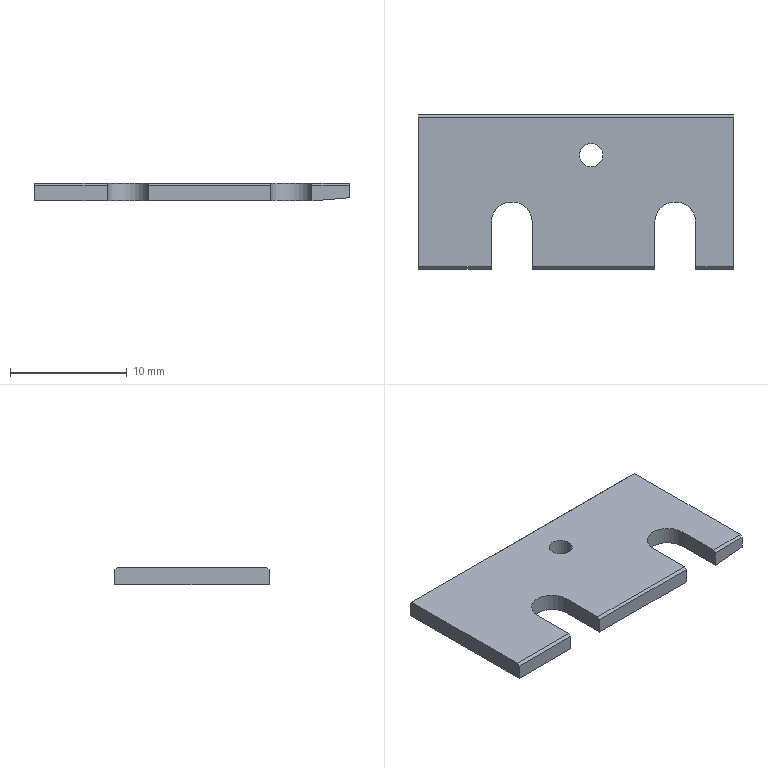Part | NX | 1 solid | 21 faces | box 27 x 13.2 x 1.5 mm | volume 467.319 mm3 | plane 17 | cylinder 4 | commonest cylinder face diameters 2 x2 3.5 x2
STEP:
#1=CARTESIAN_POINT('',(10.25,-7.3,0.75));
#2=VERTEX_POINT('',#1);
#3=CARTESIAN_POINT('',(13.5,-7.3,0.75));
#4=VERTEX_POINT('',#3);
#5=CARTESIAN_POINT('',(0.,-7.3,0.75));
#6=DIRECTION('',(1.,0.,0.));
#7=VECTOR('',#6,1000.);
#8=LINE('',#5,#7);
#9=EDGE_CURVE('',#2,#4,#8,.T.);
#10=ORIENTED_EDGE('',*,*,#9,.T.);
#11=CARTESIAN_POINT('',(13.5,5.5,0.75));
#12=VERTEX_POINT('',#11);
#13=CARTESIAN_POINT('',(13.5,0.,0.75));
#14=DIRECTION('',(0.,-1.,0.));
#15=VECTOR('',#14,1000.);
#16=LINE('',#13,#15);
#17=EDGE_CURVE('',#12,#4,#16,.T.);
#18=ORIENTED_EDGE('',*,*,#17,.F.);
#19=CARTESIAN_POINT('',(-13.5,5.5,0.75));
#20=VERTEX_POINT('',#19);
#21=CARTESIAN_POINT('',(0.,5.5,0.75));
#22=DIRECTION('',(-1.,0.,0.));
#23=VECTOR('',#22,1000.);
#24=LINE('',#21,#23);
#25=EDGE_CURVE('',#12,#20,#24,.T.);
#26=ORIENTED_EDGE('',*,*,#25,.T.);
#27=CARTESIAN_POINT('',(-13.5,-7.3,0.75));
#28=VERTEX_POINT('',#27);
#29=CARTESIAN_POINT('',(-13.5,0.,0.75));
#30=DIRECTION('',(0.,1.,0.));
#31=VECTOR('',#30,1000.);
#32=LINE('',#29,#31);
#33=EDGE_CURVE('',#28,#20,#32,.T.);
#34=ORIENTED_EDGE('',*,*,#33,.F.);
#35=CARTESIAN_POINT('',(-7.25,-7.3,0.75));
#36=VERTEX_POINT('',#35);
#37=CARTESIAN_POINT('',(0.,-7.3,0.75));
#38=DIRECTION('',(1.,0.,0.));
#39=VECTOR('',#38,1000.);
#40=LINE('',#37,#39);
#41=EDGE_CURVE('',#28,#36,#40,.T.);
#42=ORIENTED_EDGE('',*,*,#41,.T.);
#43=CARTESIAN_POINT('',(-7.25,-3.5,0.75));
#44=VERTEX_POINT('',#43);
#45=CARTESIAN_POINT('',(-7.25,0.,0.75));
#46=DIRECTION('',(0.,1.,0.));
#47=VECTOR('',#46,1000.);
#48=LINE('',#45,#47);
#49=EDGE_CURVE('',#36,#44,#48,.T.);
#50=ORIENTED_EDGE('',*,*,#49,.T.);
#51=CARTESIAN_POINT('',(-3.75,-3.5,0.75));
#52=VERTEX_POINT('',#51);
#53=CARTESIAN_POINT('',(-5.5,-3.5,0.75));
#54=DIRECTION('',(0.,0.,-1.));
#55=DIRECTION('',(-1.,0.,0.));
#56=AXIS2_PLACEMENT_3D('',#53,#54,#55);
#57=CIRCLE('',#56,1.75);
#58=EDGE_CURVE('',#44,#52,#57,.T.);
#59=ORIENTED_EDGE('',*,*,#58,.T.);
#60=CARTESIAN_POINT('',(-3.75,-7.3,0.75));
#61=VERTEX_POINT('',#60);
#62=CARTESIAN_POINT('',(-3.75,0.,0.75));
#63=DIRECTION('',(0.,-1.,0.));
#64=VECTOR('',#63,1000.);
#65=LINE('',#62,#64);
#66=EDGE_CURVE('',#52,#61,#65,.T.);
#67=ORIENTED_EDGE('',*,*,#66,.T.);
#68=CARTESIAN_POINT('',(6.75,-7.3,0.75));
#69=VERTEX_POINT('',#68);
#70=CARTESIAN_POINT('',(0.,-7.3,0.75));
#71=DIRECTION('',(1.,0.,0.));
#72=VECTOR('',#71,1000.);
#73=LINE('',#70,#72);
#74=EDGE_CURVE('',#61,#69,#73,.T.);
#75=ORIENTED_EDGE('',*,*,#74,.T.);
#76=CARTESIAN_POINT('',(6.75,-3.5,0.75));
#77=VERTEX_POINT('',#76);
#78=CARTESIAN_POINT('',(6.75,0.,0.75));
#79=DIRECTION('',(0.,1.,0.));
#80=VECTOR('',#79,1000.);
#81=LINE('',#78,#80);
#82=EDGE_CURVE('',#69,#77,#81,.T.);
#83=ORIENTED_EDGE('',*,*,#82,.T.);
#84=CARTESIAN_POINT('',(10.25,-3.5,0.75));
#85=VERTEX_POINT('',#84);
#86=CARTESIAN_POINT('',(8.5,-3.5,0.75));
#87=DIRECTION('',(0.,0.,-1.));
#88=DIRECTION('',(-1.,0.,0.));
#89=AXIS2_PLACEMENT_3D('',#86,#87,#88);
#90=CIRCLE('',#89,1.75);
#91=EDGE_CURVE('',#77,#85,#90,.T.);
#92=ORIENTED_EDGE('',*,*,#91,.T.);
#93=CARTESIAN_POINT('',(10.25,0.,0.75));
#94=DIRECTION('',(0.,-1.,0.));
#95=VECTOR('',#94,1000.);
#96=LINE('',#93,#95);
#97=EDGE_CURVE('',#85,#2,#96,.T.);
#98=ORIENTED_EDGE('',*,*,#97,.T.);
#99=EDGE_LOOP('',(#10,#18,#26,#34,#42,#50,#59,#67,#75,#83,#92,#98));
#100=FACE_BOUND('',#99,.T.);
#101=CARTESIAN_POINT('',(0.3,2.25,0.75));
#102=VERTEX_POINT('',#101);
#103=CARTESIAN_POINT('',(2.3,2.25,0.75));
#104=VERTEX_POINT('',#103);
#105=CARTESIAN_POINT('',(1.3,2.25,0.75));
#106=DIRECTION('',(0.,0.,-1.));
#107=DIRECTION('',(-1.,0.,0.));
#108=AXIS2_PLACEMENT_3D('',#105,#106,#107);
#109=CIRCLE('',#108,1.);
#110=EDGE_CURVE('',#102,#104,#109,.T.);
#111=ORIENTED_EDGE('',*,*,#110,.T.);
#112=CARTESIAN_POINT('',(1.3,2.25,0.75));
#113=DIRECTION('',(0.,0.,-1.));
#114=DIRECTION('',(-1.,0.,0.));
#115=AXIS2_PLACEMENT_3D('',#112,#113,#114);
#116=CIRCLE('',#115,1.);
#117=EDGE_CURVE('',#104,#102,#116,.T.);
#118=ORIENTED_EDGE('',*,*,#117,.T.);
#119=EDGE_LOOP('',(#111,#118));
#120=FACE_BOUND('',#119,.T.);
#121=CARTESIAN_POINT('',(0.,0.,0.75));
#122=DIRECTION('',(0.,0.,1.));
#123=DIRECTION('',(1.,0.,0.));
#124=AXIS2_PLACEMENT_3D('',#121,#122,#123);
#125=PLANE('',#124);
#126=ADVANCED_FACE('',(#100,#120),#125,.T.);
#127=CARTESIAN_POINT('',(-13.5,-7.5,-0.75));
#128=VERTEX_POINT('',#127);
#129=CARTESIAN_POINT('',(-13.5,5.7,-0.75));
#130=VERTEX_POINT('',#129);
#131=CARTESIAN_POINT('',(-13.5,0.,-0.75));
#132=DIRECTION('',(0.,1.,0.));
#133=VECTOR('',#132,1000.);
#134=LINE('',#131,#133);
#135=EDGE_CURVE('',#128,#130,#134,.T.);
#136=ORIENTED_EDGE('',*,*,#135,.F.);
#137=CARTESIAN_POINT('',(-13.5,-7.5,0.55));
#138=VERTEX_POINT('',#137);
#139=CARTESIAN_POINT('',(-13.5,-7.5,0.));
#140=DIRECTION('',(0.,0.,-1.));
#141=VECTOR('',#140,1000.);
#142=LINE('',#139,#141);
#143=EDGE_CURVE('',#138,#128,#142,.T.);
#144=ORIENTED_EDGE('',*,*,#143,.F.);
#145=CARTESIAN_POINT('',(-13.5,0.,8.05));
#146=DIRECTION('',(0.,0.7071,0.7071));
#147=VECTOR('',#146,1000.);
#148=LINE('',#145,#147);
#149=EDGE_CURVE('',#138,#28,#148,.T.);
#150=ORIENTED_EDGE('',*,*,#149,.T.);
#151=ORIENTED_EDGE('',*,*,#33,.T.);
#152=CARTESIAN_POINT('',(-13.5,5.7,0.55));
#153=VERTEX_POINT('',#152);
#154=CARTESIAN_POINT('',(-13.5,0.,6.25));
#155=DIRECTION('',(0.,0.7071,-0.7071));
#156=VECTOR('',#155,1000.);
#157=LINE('',#154,#156);
#158=EDGE_CURVE('',#20,#153,#157,.T.);
#159=ORIENTED_EDGE('',*,*,#158,.T.);
#160=CARTESIAN_POINT('',(-13.5,5.7,0.));
#161=DIRECTION('',(0.,0.,-1.));
#162=VECTOR('',#161,1000.);
#163=LINE('',#160,#162);
#164=EDGE_CURVE('',#153,#130,#163,.T.);
#165=ORIENTED_EDGE('',*,*,#164,.T.);
#166=EDGE_LOOP('',(#136,#144,#150,#151,#159,#165));
#167=FACE_BOUND('',#166,.T.);
#168=CARTESIAN_POINT('',(-13.5,7.5,-0.75));
#169=DIRECTION('',(-1.,0.,0.));
#170=DIRECTION('',(0.,0.,1.));
#171=AXIS2_PLACEMENT_3D('',#168,#169,#170);
#172=PLANE('',#171);
#173=ADVANCED_FACE('',(#167),#172,.T.);
#174=CARTESIAN_POINT('',(10.5,5.7,-0.75));
#175=VERTEX_POINT('',#174);
#176=CARTESIAN_POINT('',(0.,5.7,-0.75));
#177=DIRECTION('',(1.,0.,0.));
#178=VECTOR('',#177,1000.);
#179=LINE('',#176,#178);
#180=EDGE_CURVE('',#130,#175,#179,.T.);
#181=ORIENTED_EDGE('',*,*,#180,.F.);
#182=ORIENTED_EDGE('',*,*,#164,.F.);
#183=CARTESIAN_POINT('',(13.5,5.7,0.55));
#184=VERTEX_POINT('',#183);
#185=CARTESIAN_POINT('',(0.,5.7,0.55));
#186=DIRECTION('',(1.,0.,0.));
#187=VECTOR('',#186,1000.);
#188=LINE('',#185,#187);
#189=EDGE_CURVE('',#153,#184,#188,.T.);
#190=ORIENTED_EDGE('',*,*,#189,.T.);
#191=CARTESIAN_POINT('',(13.5,5.7,-0.4875));
#192=VERTEX_POINT('',#191);
#193=CARTESIAN_POINT('',(13.5,5.7,0.));
#194=DIRECTION('',(0.,0.,1.));
#195=VECTOR('',#194,1000.);
#196=LINE('',#193,#195);
#197=EDGE_CURVE('',#192,#184,#196,.T.);
#198=ORIENTED_EDGE('',*,*,#197,.F.);
#199=CARTESIAN_POINT('',(0.,5.7,-1.669));
#200=DIRECTION('',(0.9962,0.,0.08716));
#201=VECTOR('',#200,1000.);
#202=LINE('',#199,#201);
#203=EDGE_CURVE('',#175,#192,#202,.T.);
#204=ORIENTED_EDGE('',*,*,#203,.F.);
#205=EDGE_LOOP('',(#181,#182,#190,#198,#204));
#206=FACE_BOUND('',#205,.T.);
#207=CARTESIAN_POINT('',(13.5,5.7,-0.75));
#208=DIRECTION('',(0.,1.,0.));
#209=DIRECTION('',(1.,0.,0.));
#210=AXIS2_PLACEMENT_3D('',#207,#208,#209);
#211=PLANE('',#210);
#212=ADVANCED_FACE('',(#206),#211,.T.);
#213=CARTESIAN_POINT('',(10.5,-7.5,-0.75));
#214=VERTEX_POINT('',#213);
#215=CARTESIAN_POINT('',(10.5,0.,-0.75));
#216=DIRECTION('',(0.,-1.,0.));
#217=VECTOR('',#216,1000.);
#218=LINE('',#215,#217);
#219=EDGE_CURVE('',#175,#214,#218,.T.);
#220=ORIENTED_EDGE('',*,*,#219,.F.);
#221=ORIENTED_EDGE('',*,*,#203,.T.);
#222=CARTESIAN_POINT('',(13.5,-7.5,-0.4875));
#223=VERTEX_POINT('',#222);
#224=CARTESIAN_POINT('',(13.5,0.,-0.4875));
#225=DIRECTION('',(0.,-1.,0.));
#226=VECTOR('',#225,1000.);
#227=LINE('',#224,#226);
#228=EDGE_CURVE('',#192,#223,#227,.T.);
#229=ORIENTED_EDGE('',*,*,#228,.T.);
#230=CARTESIAN_POINT('',(0.,-7.5,-1.669));
#231=DIRECTION('',(0.9962,0.,0.08716));
#232=VECTOR('',#231,1000.);
#233=LINE('',#230,#232);
#234=EDGE_CURVE('',#214,#223,#233,.T.);
#235=ORIENTED_EDGE('',*,*,#234,.F.);
#236=EDGE_LOOP('',(#220,#221,#229,#235));
#237=FACE_BOUND('',#236,.T.);
#238=CARTESIAN_POINT('',(10.5,-7.5,-0.75));
#239=DIRECTION('',(0.08716,0.,-0.9962));
#240=DIRECTION('',(0.,-1.,0.));
#241=AXIS2_PLACEMENT_3D('',#238,#239,#240);
#242=PLANE('',#241);
#243=ADVANCED_FACE('',(#237),#242,.T.);
#244=CARTESIAN_POINT('',(-7.25,-7.5,-0.75));
#245=VERTEX_POINT('',#244);
#246=CARTESIAN_POINT('',(0.,-7.5,-0.75));
#247=DIRECTION('',(-1.,0.,0.));
#248=VECTOR('',#247,1000.);
#249=LINE('',#246,#248);
#250=EDGE_CURVE('',#245,#128,#249,.T.);
#251=ORIENTED_EDGE('',*,*,#250,.F.);
#252=CARTESIAN_POINT('',(-7.25,-7.5,0.55));
#253=VERTEX_POINT('',#252);
#254=CARTESIAN_POINT('',(-7.25,-7.5,0.));
#255=DIRECTION('',(0.,0.,-1.));
#256=VECTOR('',#255,1000.);
#257=LINE('',#254,#256);
#258=EDGE_CURVE('',#253,#245,#257,.T.);
#259=ORIENTED_EDGE('',*,*,#258,.F.);
#260=CARTESIAN_POINT('',(0.,-7.5,0.55));
#261=DIRECTION('',(-1.,0.,0.));
#262=VECTOR('',#261,1000.);
#263=LINE('',#260,#262);
#264=EDGE_CURVE('',#253,#138,#263,.T.);
#265=ORIENTED_EDGE('',*,*,#264,.T.);
#266=ORIENTED_EDGE('',*,*,#143,.T.);
#267=EDGE_LOOP('',(#251,#259,#265,#266));
#268=FACE_BOUND('',#267,.T.);
#269=CARTESIAN_POINT('',(-13.5,-7.5,-0.75));
#270=DIRECTION('',(0.,-1.,0.));
#271=DIRECTION('',(0.,0.,-1.));
#272=AXIS2_PLACEMENT_3D('',#269,#270,#271);
#273=PLANE('',#272);
#274=ADVANCED_FACE('',(#268),#273,.T.);
#275=ORIENTED_EDGE('',*,*,#135,.T.);
#276=ORIENTED_EDGE('',*,*,#180,.T.);
#277=ORIENTED_EDGE('',*,*,#219,.T.);
#278=CARTESIAN_POINT('',(10.25,-7.5,-0.75));
#279=VERTEX_POINT('',#278);
#280=CARTESIAN_POINT('',(0.,-7.5,-0.75));
#281=DIRECTION('',(-1.,0.,0.));
#282=VECTOR('',#281,1000.);
#283=LINE('',#280,#282);
#284=EDGE_CURVE('',#214,#279,#283,.T.);
#285=ORIENTED_EDGE('',*,*,#284,.T.);
#286=CARTESIAN_POINT('',(10.25,-3.5,-0.75));
#287=VERTEX_POINT('',#286);
#288=CARTESIAN_POINT('',(10.25,0.,-0.75));
#289=DIRECTION('',(0.,-1.,0.));
#290=VECTOR('',#289,1000.);
#291=LINE('',#288,#290);
#292=EDGE_CURVE('',#287,#279,#291,.T.);
#293=ORIENTED_EDGE('',*,*,#292,.F.);
#294=CARTESIAN_POINT('',(6.75,-3.5,-0.75));
#295=VERTEX_POINT('',#294);
#296=CARTESIAN_POINT('',(8.5,-3.5,-0.75));
#297=DIRECTION('',(0.,0.,-1.));
#298=DIRECTION('',(-1.,0.,0.));
#299=AXIS2_PLACEMENT_3D('',#296,#297,#298);
#300=CIRCLE('',#299,1.75);
#301=EDGE_CURVE('',#295,#287,#300,.T.);
#302=ORIENTED_EDGE('',*,*,#301,.F.);
#303=CARTESIAN_POINT('',(6.75,-7.5,-0.75));
#304=VERTEX_POINT('',#303);
#305=CARTESIAN_POINT('',(6.75,0.,-0.75));
#306=DIRECTION('',(0.,1.,0.));
#307=VECTOR('',#306,1000.);
#308=LINE('',#305,#307);
#309=EDGE_CURVE('',#304,#295,#308,.T.);
#310=ORIENTED_EDGE('',*,*,#309,.F.);
#311=CARTESIAN_POINT('',(-3.75,-7.5,-0.75));
#312=VERTEX_POINT('',#311);
#313=CARTESIAN_POINT('',(0.,-7.5,-0.75));
#314=DIRECTION('',(-1.,0.,0.));
#315=VECTOR('',#314,1000.);
#316=LINE('',#313,#315);
#317=EDGE_CURVE('',#304,#312,#316,.T.);
#318=ORIENTED_EDGE('',*,*,#317,.T.);
#319=CARTESIAN_POINT('',(-3.75,-3.5,-0.75));
#320=VERTEX_POINT('',#319);
#321=CARTESIAN_POINT('',(-3.75,0.,-0.75));
#322=DIRECTION('',(0.,-1.,0.));
#323=VECTOR('',#322,1000.);
#324=LINE('',#321,#323);
#325=EDGE_CURVE('',#320,#312,#324,.T.);
#326=ORIENTED_EDGE('',*,*,#325,.F.);
#327=CARTESIAN_POINT('',(-7.25,-3.5,-0.75));
#328=VERTEX_POINT('',#327);
#329=CARTESIAN_POINT('',(-5.5,-3.5,-0.75));
#330=DIRECTION('',(0.,0.,-1.));
#331=DIRECTION('',(-1.,0.,0.));
#332=AXIS2_PLACEMENT_3D('',#329,#330,#331);
#333=CIRCLE('',#332,1.75);
#334=EDGE_CURVE('',#328,#320,#333,.T.);
#335=ORIENTED_EDGE('',*,*,#334,.F.);
#336=CARTESIAN_POINT('',(-7.25,0.,-0.75));
#337=DIRECTION('',(0.,1.,0.));
#338=VECTOR('',#337,1000.);
#339=LINE('',#336,#338);
#340=EDGE_CURVE('',#245,#328,#339,.T.);
#341=ORIENTED_EDGE('',*,*,#340,.F.);
#342=ORIENTED_EDGE('',*,*,#250,.T.);
#343=EDGE_LOOP('',(#275,#276,#277,#285,#293,#302,#310,#318,#326,#335,#341,#342));
#344=FACE_BOUND('',#343,.T.);
#345=CARTESIAN_POINT('',(2.3,2.25,-0.75));
#346=VERTEX_POINT('',#345);
#347=CARTESIAN_POINT('',(0.3,2.25,-0.75));
#348=VERTEX_POINT('',#347);
#349=CARTESIAN_POINT('',(1.3,2.25,-0.75));
#350=DIRECTION('',(0.,0.,-1.));
#351=DIRECTION('',(-1.,0.,0.));
#352=AXIS2_PLACEMENT_3D('',#349,#350,#351);
#353=CIRCLE('',#352,1.);
#354=EDGE_CURVE('',#346,#348,#353,.T.);
#355=ORIENTED_EDGE('',*,*,#354,.F.);
#356=CARTESIAN_POINT('',(1.3,2.25,-0.75));
#357=DIRECTION('',(0.,0.,-1.));
#358=DIRECTION('',(-1.,0.,0.));
#359=AXIS2_PLACEMENT_3D('',#356,#357,#358);
#360=CIRCLE('',#359,1.);
#361=EDGE_CURVE('',#348,#346,#360,.T.);
#362=ORIENTED_EDGE('',*,*,#361,.F.);
#363=EDGE_LOOP('',(#355,#362));
#364=FACE_BOUND('',#363,.T.);
#365=CARTESIAN_POINT('',(0.,0.,-0.75));
#366=DIRECTION('',(0.,0.,1.));
#367=DIRECTION('',(1.,0.,0.));
#368=AXIS2_PLACEMENT_3D('',#365,#366,#367);
#369=PLANE('',#368);
#370=ADVANCED_FACE('',(#344,#364),#369,.F.);
#371=ORIENTED_EDGE('',*,*,#228,.F.);
#372=ORIENTED_EDGE('',*,*,#197,.T.);
#373=CARTESIAN_POINT('',(13.5,0.,6.25));
#374=DIRECTION('',(0.,-0.7071,0.7071));
#375=VECTOR('',#374,1000.);
#376=LINE('',#373,#375);
#377=EDGE_CURVE('',#184,#12,#376,.T.);
#378=ORIENTED_EDGE('',*,*,#377,.T.);
#379=ORIENTED_EDGE('',*,*,#17,.T.);
#380=CARTESIAN_POINT('',(13.5,-7.5,0.55));
#381=VERTEX_POINT('',#380);
#382=CARTESIAN_POINT('',(13.5,0.,8.05));
#383=DIRECTION('',(0.,-0.7071,-0.7071));
#384=VECTOR('',#383,1000.);
#385=LINE('',#382,#384);
#386=EDGE_CURVE('',#4,#381,#385,.T.);
#387=ORIENTED_EDGE('',*,*,#386,.T.);
#388=CARTESIAN_POINT('',(13.5,-7.5,0.));
#389=DIRECTION('',(0.,0.,1.));
#390=VECTOR('',#389,1000.);
#391=LINE('',#388,#390);
#392=EDGE_CURVE('',#223,#381,#391,.T.);
#393=ORIENTED_EDGE('',*,*,#392,.F.);
#394=EDGE_LOOP('',(#371,#372,#378,#379,#387,#393));
#395=FACE_BOUND('',#394,.T.);
#396=CARTESIAN_POINT('',(13.5,-7.5,-0.75));
#397=DIRECTION('',(1.,0.,0.));
#398=DIRECTION('',(0.,1.,0.));
#399=AXIS2_PLACEMENT_3D('',#396,#397,#398);
#400=PLANE('',#399);
#401=ADVANCED_FACE('',(#395),#400,.T.);
#402=CARTESIAN_POINT('',(10.25,-7.5,0.55));
#403=VERTEX_POINT('',#402);
#404=CARTESIAN_POINT('',(10.25,-7.5,0.));
#405=DIRECTION('',(0.,0.,1.));
#406=VECTOR('',#405,1000.);
#407=LINE('',#404,#406);
#408=EDGE_CURVE('',#279,#403,#407,.T.);
#409=ORIENTED_EDGE('',*,*,#408,.F.);
#410=ORIENTED_EDGE('',*,*,#284,.F.);
#411=ORIENTED_EDGE('',*,*,#234,.T.);
#412=ORIENTED_EDGE('',*,*,#392,.T.);
#413=CARTESIAN_POINT('',(0.,-7.5,0.55));
#414=DIRECTION('',(-1.,0.,0.));
#415=VECTOR('',#414,1000.);
#416=LINE('',#413,#415);
#417=EDGE_CURVE('',#381,#403,#416,.T.);
#418=ORIENTED_EDGE('',*,*,#417,.T.);
#419=EDGE_LOOP('',(#409,#410,#411,#412,#418));
#420=FACE_BOUND('',#419,.T.);
#421=CARTESIAN_POINT('',(-13.5,-7.5,-0.75));
#422=DIRECTION('',(0.,-1.,0.));
#423=DIRECTION('',(0.,0.,-1.));
#424=AXIS2_PLACEMENT_3D('',#421,#422,#423);
#425=PLANE('',#424);
#426=ADVANCED_FACE('',(#420),#425,.T.);
#427=ORIENTED_EDGE('',*,*,#110,.F.);
#428=CARTESIAN_POINT('',(0.3,2.25,0.75));
#429=DIRECTION('',(0.,0.,-1.));
#430=VECTOR('',#429,1000.);
#431=LINE('',#428,#430);
#432=EDGE_CURVE('',#348,#102,#431,.F.);
#433=ORIENTED_EDGE('',*,*,#432,.F.);
#434=ORIENTED_EDGE('',*,*,#361,.T.);
#435=CARTESIAN_POINT('',(2.3,2.25,0.75));
#436=DIRECTION('',(0.,0.,-1.));
#437=VECTOR('',#436,1000.);
#438=LINE('',#435,#437);
#439=EDGE_CURVE('',#346,#104,#438,.F.);
#440=ORIENTED_EDGE('',*,*,#439,.T.);
#441=EDGE_LOOP('',(#427,#433,#434,#440));
#442=FACE_BOUND('',#441,.T.);
#443=CARTESIAN_POINT('',(1.3,2.25,0.75));
#444=DIRECTION('',(0.,0.,-1.));
#445=DIRECTION('',(-1.,0.,0.));
#446=AXIS2_PLACEMENT_3D('',#443,#444,#445);
#447=CYLINDRICAL_SURFACE('',#446,1.);
#448=ADVANCED_FACE('',(#442),#447,.F.);
#449=ORIENTED_EDGE('',*,*,#301,.T.);
#450=CARTESIAN_POINT('',(10.25,-3.5,0.75));
#451=DIRECTION('',(0.,0.,-1.));
#452=VECTOR('',#451,1000.);
#453=LINE('',#450,#452);
#454=EDGE_CURVE('',#85,#287,#453,.T.);
#455=ORIENTED_EDGE('',*,*,#454,.F.);
#456=ORIENTED_EDGE('',*,*,#91,.F.);
#457=CARTESIAN_POINT('',(6.75,-3.5,0.75));
#458=DIRECTION('',(0.,0.,-1.));
#459=VECTOR('',#458,1000.);
#460=LINE('',#457,#459);
#461=EDGE_CURVE('',#77,#295,#460,.T.);
#462=ORIENTED_EDGE('',*,*,#461,.T.);
#463=EDGE_LOOP('',(#449,#455,#456,#462));
#464=FACE_BOUND('',#463,.T.);
#465=CARTESIAN_POINT('',(8.5,-3.5,0.75));
#466=DIRECTION('',(0.,0.,-1.));
#467=DIRECTION('',(-1.,0.,0.));
#468=AXIS2_PLACEMENT_3D('',#465,#466,#467);
#469=CYLINDRICAL_SURFACE('',#468,1.75);
#470=ADVANCED_FACE('',(#464),#469,.F.);
#471=CARTESIAN_POINT('',(-7.25,-3.5,0.75));
#472=DIRECTION('',(0.,0.,-1.));
#473=VECTOR('',#472,1000.);
#474=LINE('',#471,#473);
#475=EDGE_CURVE('',#44,#328,#474,.T.);
#476=ORIENTED_EDGE('',*,*,#475,.T.);
#477=ORIENTED_EDGE('',*,*,#334,.T.);
#478=CARTESIAN_POINT('',(-3.75,-3.5,0.75));
#479=DIRECTION('',(0.,0.,-1.));
#480=VECTOR('',#479,1000.);
#481=LINE('',#478,#480);
#482=EDGE_CURVE('',#52,#320,#481,.T.);
#483=ORIENTED_EDGE('',*,*,#482,.F.);
#484=ORIENTED_EDGE('',*,*,#58,.F.);
#485=EDGE_LOOP('',(#476,#477,#483,#484));
#486=FACE_BOUND('',#485,.T.);
#487=CARTESIAN_POINT('',(-5.5,-3.5,0.75));
#488=DIRECTION('',(0.,0.,-1.));
#489=DIRECTION('',(-1.,0.,0.));
#490=AXIS2_PLACEMENT_3D('',#487,#488,#489);
#491=CYLINDRICAL_SURFACE('',#490,1.75);
#492=ADVANCED_FACE('',(#486),#491,.F.);
#493=CARTESIAN_POINT('',(6.75,-7.5,0.55));
#494=VERTEX_POINT('',#493);
#495=CARTESIAN_POINT('',(6.75,-7.5,0.));
#496=DIRECTION('',(0.,0.,-1.));
#497=VECTOR('',#496,1000.);
#498=LINE('',#495,#497);
#499=EDGE_CURVE('',#494,#304,#498,.T.);
#500=ORIENTED_EDGE('',*,*,#499,.F.);
#501=CARTESIAN_POINT('',(-3.75,-7.5,0.55));
#502=VERTEX_POINT('',#501);
#503=CARTESIAN_POINT('',(0.,-7.5,0.55));
#504=DIRECTION('',(-1.,0.,0.));
#505=VECTOR('',#504,1000.);
#506=LINE('',#503,#505);
#507=EDGE_CURVE('',#494,#502,#506,.T.);
#508=ORIENTED_EDGE('',*,*,#507,.T.);
#509=CARTESIAN_POINT('',(-3.75,-7.5,0.));
#510=DIRECTION('',(0.,0.,1.));
#511=VECTOR('',#510,1000.);
#512=LINE('',#509,#511);
#513=EDGE_CURVE('',#312,#502,#512,.T.);
#514=ORIENTED_EDGE('',*,*,#513,.F.);
#515=ORIENTED_EDGE('',*,*,#317,.F.);
#516=EDGE_LOOP('',(#500,#508,#514,#515));
#517=FACE_BOUND('',#516,.T.);
#518=CARTESIAN_POINT('',(-13.5,-7.5,-0.75));
#519=DIRECTION('',(0.,-1.,0.));
#520=DIRECTION('',(0.,0.,-1.));
#521=AXIS2_PLACEMENT_3D('',#518,#519,#520);
#522=PLANE('',#521);
#523=ADVANCED_FACE('',(#517),#522,.T.);
#524=ORIENTED_EDGE('',*,*,#292,.T.);
#525=ORIENTED_EDGE('',*,*,#408,.T.);
#526=CARTESIAN_POINT('',(10.25,0.,8.05));
#527=DIRECTION('',(0.,-0.7071,-0.7071));
#528=VECTOR('',#527,1000.);
#529=LINE('',#526,#528);
#530=EDGE_CURVE('',#2,#403,#529,.T.);
#531=ORIENTED_EDGE('',*,*,#530,.F.);
#532=ORIENTED_EDGE('',*,*,#97,.F.);
#533=ORIENTED_EDGE('',*,*,#454,.T.);
#534=EDGE_LOOP('',(#524,#525,#531,#532,#533));
#535=FACE_BOUND('',#534,.T.);
#536=CARTESIAN_POINT('',(10.25,-3.5,-0.9));
#537=DIRECTION('',(1.,0.,0.));
#538=DIRECTION('',(0.,1.,0.));
#539=AXIS2_PLACEMENT_3D('',#536,#537,#538);
#540=PLANE('',#539);
#541=ADVANCED_FACE('',(#535),#540,.F.);
#542=ORIENTED_EDGE('',*,*,#82,.F.);
#543=CARTESIAN_POINT('',(6.75,0.,8.05));
#544=DIRECTION('',(0.,0.7071,0.7071));
#545=VECTOR('',#544,1000.);
#546=LINE('',#543,#545);
#547=EDGE_CURVE('',#494,#69,#546,.T.);
#548=ORIENTED_EDGE('',*,*,#547,.F.);
#549=ORIENTED_EDGE('',*,*,#499,.T.);
#550=ORIENTED_EDGE('',*,*,#309,.T.);
#551=ORIENTED_EDGE('',*,*,#461,.F.);
#552=EDGE_LOOP('',(#542,#548,#549,#550,#551));
#553=FACE_BOUND('',#552,.T.);
#554=CARTESIAN_POINT('',(6.75,-10.6,-0.9));
#555=DIRECTION('',(-1.,0.,0.));
#556=DIRECTION('',(0.,0.,1.));
#557=AXIS2_PLACEMENT_3D('',#554,#555,#556);
#558=PLANE('',#557);
#559=ADVANCED_FACE('',(#553),#558,.F.);
#560=ORIENTED_EDGE('',*,*,#513,.T.);
#561=CARTESIAN_POINT('',(-3.75,0.,8.05));
#562=DIRECTION('',(0.,-0.7071,-0.7071));
#563=VECTOR('',#562,1000.);
#564=LINE('',#561,#563);
#565=EDGE_CURVE('',#61,#502,#564,.T.);
#566=ORIENTED_EDGE('',*,*,#565,.F.);
#567=ORIENTED_EDGE('',*,*,#66,.F.);
#568=ORIENTED_EDGE('',*,*,#482,.T.);
#569=ORIENTED_EDGE('',*,*,#325,.T.);
#570=EDGE_LOOP('',(#560,#566,#567,#568,#569));
#571=FACE_BOUND('',#570,.T.);
#572=CARTESIAN_POINT('',(-3.75,-3.5,-0.9));
#573=DIRECTION('',(1.,0.,0.));
#574=DIRECTION('',(0.,1.,0.));
#575=AXIS2_PLACEMENT_3D('',#572,#573,#574);
#576=PLANE('',#575);
#577=ADVANCED_FACE('',(#571),#576,.F.);
#578=ORIENTED_EDGE('',*,*,#258,.T.);
#579=ORIENTED_EDGE('',*,*,#340,.T.);
#580=ORIENTED_EDGE('',*,*,#475,.F.);
#581=ORIENTED_EDGE('',*,*,#49,.F.);
#582=CARTESIAN_POINT('',(-7.25,0.,8.05));
#583=DIRECTION('',(0.,0.7071,0.7071));
#584=VECTOR('',#583,1000.);
#585=LINE('',#582,#584);
#586=EDGE_CURVE('',#253,#36,#585,.T.);
#587=ORIENTED_EDGE('',*,*,#586,.F.);
#588=EDGE_LOOP('',(#578,#579,#580,#581,#587));
#589=FACE_BOUND('',#588,.T.);
#590=CARTESIAN_POINT('',(-7.25,-11.4,-0.9));
#591=DIRECTION('',(-1.,0.,0.));
#592=DIRECTION('',(0.,0.,1.));
#593=AXIS2_PLACEMENT_3D('',#590,#591,#592);
#594=PLANE('',#593);
#595=ADVANCED_FACE('',(#589),#594,.F.);
#596=ORIENTED_EDGE('',*,*,#25,.F.);
#597=ORIENTED_EDGE('',*,*,#377,.F.);
#598=ORIENTED_EDGE('',*,*,#189,.F.);
#599=ORIENTED_EDGE('',*,*,#158,.F.);
#600=EDGE_LOOP('',(#596,#597,#598,#599));
#601=FACE_BOUND('',#600,.T.);
#602=CARTESIAN_POINT('',(0.,5.6,0.65));
#603=DIRECTION('',(0.,-0.7071,-0.7071));
#604=DIRECTION('',(0.,-0.7071,0.7071));
#605=AXIS2_PLACEMENT_3D('',#602,#603,#604);
#606=PLANE('',#605);
#607=ADVANCED_FACE('',(#601),#606,.F.);
#608=ORIENTED_EDGE('',*,*,#41,.F.);
#609=ORIENTED_EDGE('',*,*,#149,.F.);
#610=ORIENTED_EDGE('',*,*,#264,.F.);
#611=ORIENTED_EDGE('',*,*,#586,.T.);
#612=EDGE_LOOP('',(#608,#609,#610,#611));
#613=FACE_BOUND('',#612,.T.);
#614=CARTESIAN_POINT('',(-10.375,-7.4,0.65));
#615=DIRECTION('',(0.,0.7071,-0.7071));
#616=DIRECTION('',(-1.,0.,0.));
#617=AXIS2_PLACEMENT_3D('',#614,#615,#616);
#618=PLANE('',#617);
#619=ADVANCED_FACE('',(#613),#618,.F.);
#620=ORIENTED_EDGE('',*,*,#74,.F.);
#621=ORIENTED_EDGE('',*,*,#565,.T.);
#622=ORIENTED_EDGE('',*,*,#507,.F.);
#623=ORIENTED_EDGE('',*,*,#547,.T.);
#624=EDGE_LOOP('',(#620,#621,#622,#623));
#625=FACE_BOUND('',#624,.T.);
#626=CARTESIAN_POINT('',(1.5,-7.4,0.65));
#627=DIRECTION('',(0.,0.7071,-0.7071));
#628=DIRECTION('',(-1.,0.,0.));
#629=AXIS2_PLACEMENT_3D('',#626,#627,#628);
#630=PLANE('',#629);
#631=ADVANCED_FACE('',(#625),#630,.F.);
#632=ORIENTED_EDGE('',*,*,#9,.F.);
#633=ORIENTED_EDGE('',*,*,#530,.T.);
#634=ORIENTED_EDGE('',*,*,#417,.F.);
#635=ORIENTED_EDGE('',*,*,#386,.F.);
#636=EDGE_LOOP('',(#632,#633,#634,#635));
#637=FACE_BOUND('',#636,.T.);
#638=CARTESIAN_POINT('',(11.875,-7.4,0.65));
#639=DIRECTION('',(0.,0.7071,-0.7071));
#640=DIRECTION('',(-1.,0.,0.));
#641=AXIS2_PLACEMENT_3D('',#638,#639,#640);
#642=PLANE('',#641);
#643=ADVANCED_FACE('',(#637),#642,.F.);
#644=ORIENTED_EDGE('',*,*,#354,.T.);
#645=ORIENTED_EDGE('',*,*,#432,.T.);
#646=ORIENTED_EDGE('',*,*,#117,.F.);
#647=ORIENTED_EDGE('',*,*,#439,.F.);
#648=EDGE_LOOP('',(#644,#645,#646,#647));
#649=FACE_BOUND('',#648,.T.);
#650=CARTESIAN_POINT('',(1.3,2.25,0.75));
#651=DIRECTION('',(0.,0.,-1.));
#652=DIRECTION('',(-1.,0.,0.));
#653=AXIS2_PLACEMENT_3D('',#650,#651,#652);
#654=CYLINDRICAL_SURFACE('',#653,1.);
#655=ADVANCED_FACE('',(#649),#654,.F.);
#656=CLOSED_SHELL('',(#126,#173,#212,#243,#274,#370,#401,#426,#448,#470,#492,#523,#541,#559,#577,#595,#607,#619,#631,#643,#655));
#657=MANIFOLD_SOLID_BREP('',#656);
#658=(LENGTH_UNIT()NAMED_UNIT(*)SI_UNIT(.MILLI.,.METRE.));
#659=UNCERTAINTY_MEASURE_WITH_UNIT(LENGTH_MEASURE(0.00001),#658,'','');
#660=(NAMED_UNIT(*)PLANE_ANGLE_UNIT()SI_UNIT($,.RADIAN.));
#661=(NAMED_UNIT(*)SI_UNIT($,.STERADIAN.)SOLID_ANGLE_UNIT());
#662=(GEOMETRIC_REPRESENTATION_CONTEXT(3)GLOBAL_UNCERTAINTY_ASSIGNED_CONTEXT((#659))GLOBAL_UNIT_ASSIGNED_CONTEXT((#658,#660,#661))REPRESENTATION_CONTEXT('',''));
#663=ADVANCED_BREP_SHAPE_REPRESENTATION('',(#657),#662);